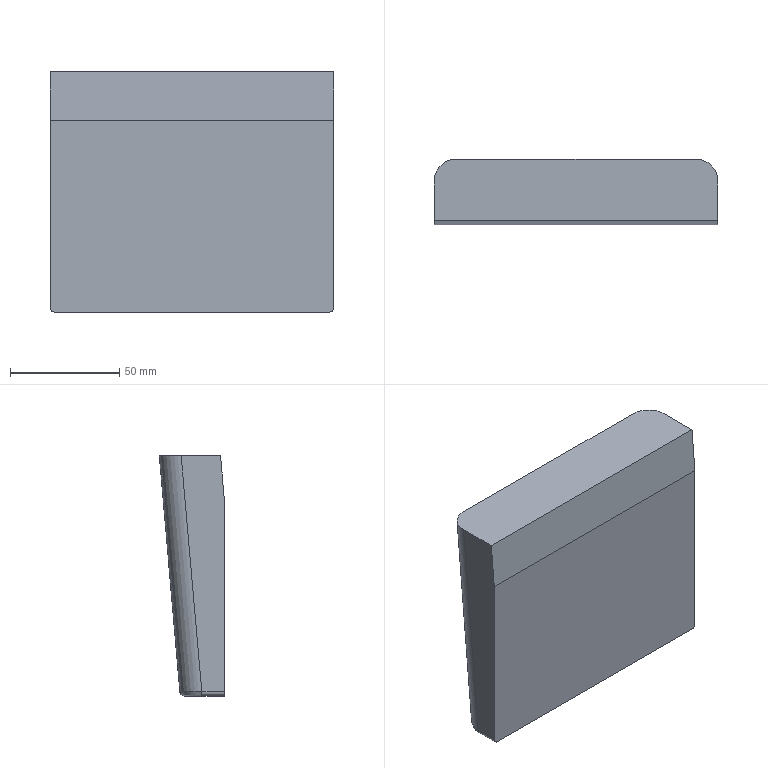Part | STEP file | 4-20.sldasm-Part-379 | 1 solid | 14 faces | box 130 x 29.992 x 110 mm | volume 352459 mm3 | plane 7 | cylinder 5 | spline 2 | commonest cylinder face diameters 4 x3 20 x2
STEP:
#1=CARTESIAN_POINT('',(65.,431.929,150.));
#2=VERTEX_POINT('',#1);
#3=CARTESIAN_POINT('',(65.,449.954,150.));
#4=VERTEX_POINT('',#3);
#5=CARTESIAN_POINT('',(65.,430.,150.));
#6=DIRECTION('',(0.,1.,0.));
#7=VECTOR('',#6,1000.);
#8=LINE('',#5,#7);
#9=EDGE_CURVE('',#2,#4,#8,.T.);
#10=ORIENTED_EDGE('',*,*,#9,.F.);
#11=CARTESIAN_POINT('',(65.,430.,127.947));
#12=VERTEX_POINT('',#11);
#13=CARTESIAN_POINT('',(65.,440.597,249.073));
#14=DIRECTION('',(0.,-0.08716,-0.9962));
#15=VECTOR('',#14,1000.);
#16=LINE('',#13,#15);
#17=EDGE_CURVE('',#2,#12,#16,.T.);
#18=ORIENTED_EDGE('',*,*,#17,.T.);
#19=CARTESIAN_POINT('',(65.,430.,42.));
#20=VERTEX_POINT('',#19);
#21=CARTESIAN_POINT('',(65.,430.,250.));
#22=DIRECTION('',(0.,0.,-1.));
#23=VECTOR('',#22,1000.);
#24=LINE('',#21,#23);
#25=EDGE_CURVE('',#12,#20,#24,.T.);
#26=ORIENTED_EDGE('',*,*,#25,.T.);
#27=CARTESIAN_POINT('',(65.,440.505,42.));
#28=VERTEX_POINT('',#27);
#29=CARTESIAN_POINT('',(65.,430.,42.));
#30=DIRECTION('',(0.,1.,0.));
#31=VECTOR('',#30,1000.);
#32=LINE('',#29,#31);
#33=EDGE_CURVE('',#20,#28,#32,.T.);
#34=ORIENTED_EDGE('',*,*,#33,.T.);
#35=CARTESIAN_POINT('',(65.,458.485,247.508));
#36=DIRECTION('',(0.,0.08716,0.9962));
#37=VECTOR('',#36,1000.);
#38=LINE('',#35,#37);
#39=EDGE_CURVE('',#28,#4,#38,.T.);
#40=ORIENTED_EDGE('',*,*,#39,.T.);
#41=EDGE_LOOP('',(#10,#18,#26,#34,#40));
#42=FACE_OUTER_BOUND('',#41,.T.);
#43=CARTESIAN_POINT('',(65.,430.,250.));
#44=DIRECTION('',(-1.,0.,0.));
#45=DIRECTION('',(0.,0.,1.));
#46=AXIS2_PLACEMENT_3D('',#43,#44,#45);
#47=PLANE('',#46);
#48=ADVANCED_FACE('',(#42),#47,.F.);
#49=CARTESIAN_POINT('',(55.,459.992,150.));
#50=VERTEX_POINT('',#49);
#51=CARTESIAN_POINT('',(55.,450.528,41.826));
#52=VERTEX_POINT('',#51);
#53=CARTESIAN_POINT('',(55.,460.008,150.174));
#54=DIRECTION('',(0.,-0.08716,-0.9962));
#55=VECTOR('',#54,1000.);
#56=LINE('',#53,#55);
#57=EDGE_CURVE('',#50,#52,#56,.T.);
#58=ORIENTED_EDGE('',*,*,#57,.T.);
#59=CARTESIAN_POINT('',(-55.,450.528,41.826));
#60=VERTEX_POINT('',#59);
#61=CARTESIAN_POINT('',(55.,450.528,41.826));
#62=DIRECTION('',(-1.,0.,0.));
#63=VECTOR('',#62,1000.);
#64=LINE('',#61,#63);
#65=EDGE_CURVE('',#52,#60,#64,.T.);
#66=ORIENTED_EDGE('',*,*,#65,.T.);
#67=CARTESIAN_POINT('',(-55.,459.992,150.));
#68=VERTEX_POINT('',#67);
#69=CARTESIAN_POINT('',(-55.,460.008,150.174));
#70=DIRECTION('',(0.,0.08716,0.9962));
#71=VECTOR('',#70,1000.);
#72=LINE('',#69,#71);
#73=EDGE_CURVE('',#60,#68,#72,.T.);
#74=ORIENTED_EDGE('',*,*,#73,.T.);
#75=CARTESIAN_POINT('',(55.,459.992,150.));
#76=DIRECTION('',(-1.,0.,0.));
#77=VECTOR('',#76,1000.);
#78=LINE('',#75,#77);
#79=EDGE_CURVE('',#50,#68,#78,.T.);
#80=ORIENTED_EDGE('',*,*,#79,.F.);
#81=EDGE_LOOP('',(#58,#66,#74,#80));
#82=FACE_OUTER_BOUND('',#81,.T.);
#83=CARTESIAN_POINT('',(55.,460.008,150.174));
#84=DIRECTION('',(0.,-0.9962,0.08716));
#85=DIRECTION('',(0.,-0.08716,-0.9962));
#86=AXIS2_PLACEMENT_3D('',#83,#84,#85);
#87=PLANE('',#86);
#88=ADVANCED_FACE('',(#82),#87,.F.);
#89=CARTESIAN_POINT('',(-65.,430.,127.947));
#90=VERTEX_POINT('',#89);
#91=CARTESIAN_POINT('',(-65.,430.,42.));
#92=VERTEX_POINT('',#91);
#93=CARTESIAN_POINT('',(-65.,430.,250.));
#94=DIRECTION('',(0.,0.,-1.));
#95=VECTOR('',#94,1000.);
#96=LINE('',#93,#95);
#97=EDGE_CURVE('',#90,#92,#96,.T.);
#98=ORIENTED_EDGE('',*,*,#97,.F.);
#99=CARTESIAN_POINT('',(-65.,431.929,150.));
#100=VERTEX_POINT('',#99);
#101=CARTESIAN_POINT('',(-65.,440.764,250.983));
#102=DIRECTION('',(0.,0.08716,0.9962));
#103=VECTOR('',#102,1000.);
#104=LINE('',#101,#103);
#105=EDGE_CURVE('',#90,#100,#104,.T.);
#106=ORIENTED_EDGE('',*,*,#105,.T.);
#107=CARTESIAN_POINT('',(-65.,449.954,150.));
#108=VERTEX_POINT('',#107);
#109=CARTESIAN_POINT('',(-65.,452.,150.));
#110=DIRECTION('',(0.,-1.,0.));
#111=VECTOR('',#110,1000.);
#112=LINE('',#109,#111);
#113=EDGE_CURVE('',#108,#100,#112,.T.);
#114=ORIENTED_EDGE('',*,*,#113,.F.);
#115=CARTESIAN_POINT('',(-65.,440.505,42.));
#116=VERTEX_POINT('',#115);
#117=CARTESIAN_POINT('',(-65.,458.652,249.418));
#118=DIRECTION('',(0.,-0.08716,-0.9962));
#119=VECTOR('',#118,1000.);
#120=LINE('',#117,#119);
#121=EDGE_CURVE('',#108,#116,#120,.T.);
#122=ORIENTED_EDGE('',*,*,#121,.T.);
#123=CARTESIAN_POINT('',(-65.,452.,42.));
#124=DIRECTION('',(0.,-1.,0.));
#125=VECTOR('',#124,1000.);
#126=LINE('',#123,#125);
#127=EDGE_CURVE('',#116,#92,#126,.T.);
#128=ORIENTED_EDGE('',*,*,#127,.T.);
#129=EDGE_LOOP('',(#98,#106,#114,#122,#128));
#130=FACE_OUTER_BOUND('',#129,.T.);
#131=CARTESIAN_POINT('',(-65.,452.,250.));
#132=DIRECTION('',(1.,0.,0.));
#133=DIRECTION('',(0.,0.,-1.));
#134=AXIS2_PLACEMENT_3D('',#131,#132,#133);
#135=PLANE('',#134);
#136=ADVANCED_FACE('',(#130),#135,.F.);
#137=ORIENTED_EDGE('',*,*,#25,.F.);
#138=CARTESIAN_POINT('',(-65.,430.,127.947));
#139=DIRECTION('',(-1.,0.,0.));
#140=VECTOR('',#139,1000.);
#141=LINE('',#138,#140);
#142=EDGE_CURVE('',#12,#90,#141,.T.);
#143=ORIENTED_EDGE('',*,*,#142,.T.);
#144=ORIENTED_EDGE('',*,*,#97,.T.);
#145=CARTESIAN_POINT('',(-63.,430.,40.));
#146=VERTEX_POINT('',#145);
#147=CARTESIAN_POINT('',(-63.,430.,42.));
#148=DIRECTION('',(0.,-1.,0.));
#149=DIRECTION('',(0.,0.,1.));
#150=AXIS2_PLACEMENT_3D('',#147,#148,#149);
#151=CIRCLE('',#150,2.);
#152=EDGE_CURVE('',#92,#146,#151,.T.);
#153=ORIENTED_EDGE('',*,*,#152,.T.);
#154=CARTESIAN_POINT('',(63.,430.,40.));
#155=VERTEX_POINT('',#154);
#156=CARTESIAN_POINT('',(-65.,430.,40.));
#157=DIRECTION('',(1.,0.,0.));
#158=VECTOR('',#157,1000.);
#159=LINE('',#156,#158);
#160=EDGE_CURVE('',#146,#155,#159,.T.);
#161=ORIENTED_EDGE('',*,*,#160,.T.);
#162=CARTESIAN_POINT('',(63.,430.,42.));
#163=DIRECTION('',(0.,-1.,0.));
#164=DIRECTION('',(0.,0.,1.));
#165=AXIS2_PLACEMENT_3D('',#162,#163,#164);
#166=CIRCLE('',#165,2.);
#167=EDGE_CURVE('',#155,#20,#166,.T.);
#168=ORIENTED_EDGE('',*,*,#167,.T.);
#169=EDGE_LOOP('',(#137,#143,#144,#153,#161,#168));
#170=FACE_OUTER_BOUND('',#169,.T.);
#171=CARTESIAN_POINT('',(-65.,430.,250.));
#172=DIRECTION('',(0.,1.,0.));
#173=DIRECTION('',(0.,0.,1.));
#174=AXIS2_PLACEMENT_3D('',#171,#172,#173);
#175=PLANE('',#174);
#176=ADVANCED_FACE('',(#170),#175,.F.);
#177=CARTESIAN_POINT('',(95.,431.929,150.));
#178=DIRECTION('',(-1.,0.,0.));
#179=VECTOR('',#178,1000.);
#180=LINE('',#177,#179);
#181=EDGE_CURVE('',#2,#100,#180,.T.);
#182=ORIENTED_EDGE('',*,*,#181,.F.);
#183=ORIENTED_EDGE('',*,*,#9,.T.);
#184=CARTESIAN_POINT('',(65.,449.954,150.));
#185=CARTESIAN_POINT('',(65.,455.834,150.));
#186=CARTESIAN_POINT('',(60.858,459.992,150.));
#187=CARTESIAN_POINT('',(55.,459.992,150.));
#188=(BOUNDED_CURVE()B_SPLINE_CURVE(3,(#184,#185,#186,#187),.UNSPECIFIED.,.F.,.T.)B_SPLINE_CURVE_WITH_KNOTS((4,4),(1.571,3.142),.UNSPECIFIED.)CURVE()GEOMETRIC_REPRESENTATION_ITEM()RATIONAL_B_SPLINE_CURVE((1.,0.8047,0.8047,1.))REPRESENTATION_ITEM(''));
#189=EDGE_CURVE('',#4,#50,#188,.T.);
#190=ORIENTED_EDGE('',*,*,#189,.T.);
#191=ORIENTED_EDGE('',*,*,#79,.T.);
#192=CARTESIAN_POINT('',(-55.,459.992,150.));
#193=CARTESIAN_POINT('',(-60.858,459.992,150.));
#194=CARTESIAN_POINT('',(-65.,455.834,150.));
#195=CARTESIAN_POINT('',(-65.,449.954,150.));
#196=(BOUNDED_CURVE()B_SPLINE_CURVE(3,(#192,#193,#194,#195),.UNSPECIFIED.,.F.,.F.)B_SPLINE_CURVE_WITH_KNOTS((4,4),(3.142,4.712),.UNSPECIFIED.)CURVE()GEOMETRIC_REPRESENTATION_ITEM()RATIONAL_B_SPLINE_CURVE((1.,0.8047,0.8047,1.))REPRESENTATION_ITEM(''));
#197=EDGE_CURVE('',#68,#108,#196,.T.);
#198=ORIENTED_EDGE('',*,*,#197,.T.);
#199=ORIENTED_EDGE('',*,*,#113,.T.);
#200=EDGE_LOOP('',(#182,#183,#190,#191,#198,#199));
#201=FACE_OUTER_BOUND('',#200,.T.);
#202=CARTESIAN_POINT('',(-100.,17.,150.));
#203=DIRECTION('',(0.,0.,-1.));
#204=DIRECTION('',(-1.,0.,0.));
#205=AXIS2_PLACEMENT_3D('',#202,#203,#204);
#206=PLANE('',#205);
#207=ADVANCED_FACE('',(#201),#206,.F.);
#208=CARTESIAN_POINT('',(55.,448.536,40.));
#209=VERTEX_POINT('',#208);
#210=CARTESIAN_POINT('',(63.,440.505,40.));
#211=VERTEX_POINT('',#210);
#212=CARTESIAN_POINT('',(55.,448.536,40.));
#213=CARTESIAN_POINT('',(59.686,448.536,40.));
#214=CARTESIAN_POINT('',(63.,445.21,40.));
#215=CARTESIAN_POINT('',(63.,440.505,40.));
#216=(BOUNDED_CURVE()B_SPLINE_CURVE(3,(#212,#213,#214,#215),.UNSPECIFIED.,.F.,.T.)B_SPLINE_CURVE_WITH_KNOTS((4,4),(3.142,4.712),.UNSPECIFIED.)CURVE()GEOMETRIC_REPRESENTATION_ITEM()RATIONAL_B_SPLINE_CURVE((1.,0.8047,0.8047,1.))REPRESENTATION_ITEM(''));
#217=EDGE_CURVE('',#209,#211,#216,.T.);
#218=ORIENTED_EDGE('',*,*,#217,.T.);
#219=CARTESIAN_POINT('',(63.,17.,40.));
#220=DIRECTION('',(0.,-1.,0.));
#221=VECTOR('',#220,1000.);
#222=LINE('',#219,#221);
#223=EDGE_CURVE('',#211,#155,#222,.T.);
#224=ORIENTED_EDGE('',*,*,#223,.T.);
#225=ORIENTED_EDGE('',*,*,#160,.F.);
#226=CARTESIAN_POINT('',(-63.,440.505,40.));
#227=VERTEX_POINT('',#226);
#228=CARTESIAN_POINT('',(-63.,17.,40.));
#229=DIRECTION('',(0.,1.,0.));
#230=VECTOR('',#229,1000.);
#231=LINE('',#228,#230);
#232=EDGE_CURVE('',#146,#227,#231,.T.);
#233=ORIENTED_EDGE('',*,*,#232,.T.);
#234=CARTESIAN_POINT('',(-55.,448.536,40.));
#235=VERTEX_POINT('',#234);
#236=CARTESIAN_POINT('',(-63.,440.505,40.));
#237=CARTESIAN_POINT('',(-63.,445.21,40.));
#238=CARTESIAN_POINT('',(-59.686,448.536,40.));
#239=CARTESIAN_POINT('',(-55.,448.536,40.));
#240=(BOUNDED_CURVE()B_SPLINE_CURVE(3,(#236,#237,#238,#239),.UNSPECIFIED.,.F.,.F.)B_SPLINE_CURVE_WITH_KNOTS((4,4),(1.571,3.142),.UNSPECIFIED.)CURVE()GEOMETRIC_REPRESENTATION_ITEM()RATIONAL_B_SPLINE_CURVE((1.,0.8047,0.8047,1.))REPRESENTATION_ITEM(''));
#241=EDGE_CURVE('',#227,#235,#240,.T.);
#242=ORIENTED_EDGE('',*,*,#241,.T.);
#243=CARTESIAN_POINT('',(100.,448.536,40.));
#244=DIRECTION('',(1.,0.,0.));
#245=VECTOR('',#244,1000.);
#246=LINE('',#243,#245);
#247=EDGE_CURVE('',#235,#209,#246,.T.);
#248=ORIENTED_EDGE('',*,*,#247,.T.);
#249=EDGE_LOOP('',(#218,#224,#225,#233,#242,#248));
#250=FACE_OUTER_BOUND('',#249,.T.);
#251=CARTESIAN_POINT('',(100.,17.,40.));
#252=DIRECTION('',(0.,0.,-1.));
#253=DIRECTION('',(-1.,0.,0.));
#254=AXIS2_PLACEMENT_3D('',#251,#252,#253);
#255=PLANE('',#254);
#256=ADVANCED_FACE('',(#250),#255,.T.);
#257=ORIENTED_EDGE('',*,*,#73,.F.);
#258=CARTESIAN_POINT('',(-55.,450.528,41.826));
#259=CARTESIAN_POINT('',(-60.858,450.528,41.826));
#260=CARTESIAN_POINT('',(-65.,446.377,41.898));
#261=CARTESIAN_POINT('',(-65.,440.505,42.));
#262=(BOUNDED_CURVE()B_SPLINE_CURVE(3,(#258,#259,#260,#261),.UNSPECIFIED.,.F.,.T.)B_SPLINE_CURVE_WITH_KNOTS((4,4),(3.142,4.712),.UNSPECIFIED.)CURVE()GEOMETRIC_REPRESENTATION_ITEM()RATIONAL_B_SPLINE_CURVE((1.,0.8047,0.8047,1.))REPRESENTATION_ITEM(''));
#263=EDGE_CURVE('',#60,#116,#262,.T.);
#264=ORIENTED_EDGE('',*,*,#263,.T.);
#265=ORIENTED_EDGE('',*,*,#121,.F.);
#266=ORIENTED_EDGE('',*,*,#197,.F.);
#267=EDGE_LOOP('',(#257,#264,#265,#266));
#268=FACE_OUTER_BOUND('',#267,.T.);
#269=CARTESIAN_POINT('',(-55.,458.652,249.418));
#270=DIRECTION('',(0.,-0.08716,-0.9962));
#271=DIRECTION('',(0.,0.9962,-0.08716));
#272=AXIS2_PLACEMENT_3D('',#269,#270,#271);
#273=CYLINDRICAL_SURFACE('',#272,10.);
#274=ADVANCED_FACE('',(#268),#273,.T.);
#275=ORIENTED_EDGE('',*,*,#39,.F.);
#276=CARTESIAN_POINT('',(65.,440.505,42.));
#277=CARTESIAN_POINT('',(65.,446.377,41.898));
#278=CARTESIAN_POINT('',(60.858,450.528,41.826));
#279=CARTESIAN_POINT('',(55.,450.528,41.826));
#280=(BOUNDED_CURVE()B_SPLINE_CURVE(3,(#276,#277,#278,#279),.UNSPECIFIED.,.F.,.F.)B_SPLINE_CURVE_WITH_KNOTS((4,4),(1.571,3.142),.UNSPECIFIED.)CURVE()GEOMETRIC_REPRESENTATION_ITEM()RATIONAL_B_SPLINE_CURVE((1.,0.8047,0.8047,1.))REPRESENTATION_ITEM(''));
#281=EDGE_CURVE('',#28,#52,#280,.T.);
#282=ORIENTED_EDGE('',*,*,#281,.T.);
#283=ORIENTED_EDGE('',*,*,#57,.F.);
#284=ORIENTED_EDGE('',*,*,#189,.F.);
#285=EDGE_LOOP('',(#275,#282,#283,#284));
#286=FACE_OUTER_BOUND('',#285,.T.);
#287=CARTESIAN_POINT('',(55.,450.046,151.046));
#288=DIRECTION('',(0.,-0.08716,-0.9962));
#289=DIRECTION('',(0.,0.9962,-0.08716));
#290=AXIS2_PLACEMENT_3D('',#287,#288,#289);
#291=CYLINDRICAL_SURFACE('',#290,10.);
#292=ADVANCED_FACE('',(#286),#291,.T.);
#293=ORIENTED_EDGE('',*,*,#152,.F.);
#294=ORIENTED_EDGE('',*,*,#127,.F.);
#295=CARTESIAN_POINT('',(-63.,440.505,42.));
#296=DIRECTION('',(0.,1.,0.));
#297=DIRECTION('',(0.,0.,1.));
#298=AXIS2_PLACEMENT_3D('',#295,#296,#297);
#299=CIRCLE('',#298,2.);
#300=EDGE_CURVE('',#227,#116,#299,.T.);
#301=ORIENTED_EDGE('',*,*,#300,.F.);
#302=ORIENTED_EDGE('',*,*,#232,.F.);
#303=EDGE_LOOP('',(#293,#294,#301,#302));
#304=FACE_OUTER_BOUND('',#303,.T.);
#305=CARTESIAN_POINT('',(-63.,452.,42.));
#306=DIRECTION('',(0.,1.,0.));
#307=DIRECTION('',(0.,0.,1.));
#308=AXIS2_PLACEMENT_3D('',#305,#306,#307);
#309=CYLINDRICAL_SURFACE('',#308,2.);
#310=ADVANCED_FACE('',(#304),#309,.T.);
#311=ORIENTED_EDGE('',*,*,#300,.T.);
#312=ORIENTED_EDGE('',*,*,#263,.F.);
#313=CARTESIAN_POINT('',(-55.,448.536,42.));
#314=DIRECTION('',(1.,0.,0.));
#315=DIRECTION('',(0.,0.,-1.));
#316=AXIS2_PLACEMENT_3D('',#313,#314,#315);
#317=CIRCLE('',#316,2.);
#318=EDGE_CURVE('',#235,#60,#317,.T.);
#319=ORIENTED_EDGE('',*,*,#318,.F.);
#320=ORIENTED_EDGE('',*,*,#241,.F.);
#321=EDGE_LOOP('',(#311,#312,#319,#320));
#322=FACE_OUTER_BOUND('',#321,.T.);
#323=CARTESIAN_POINT('',(-65.,440.505,42.));
#324=CARTESIAN_POINT('',(-65.,440.505,40.));
#325=CARTESIAN_POINT('',(-63.,440.505,40.));
#326=CARTESIAN_POINT('',(-65.,441.818,41.977));
#327=CARTESIAN_POINT('',(-64.977,441.81,40.));
#328=CARTESIAN_POINT('',(-63.,441.557,40.));
#329=CARTESIAN_POINT('',(-64.74,443.129,41.954));
#330=CARTESIAN_POINT('',(-64.698,443.113,40.));
#331=CARTESIAN_POINT('',(-62.792,442.607,40.));
#332=CARTESIAN_POINT('',(-63.738,445.553,41.912));
#333=CARTESIAN_POINT('',(-63.666,445.507,40.));
#334=CARTESIAN_POINT('',(-61.99,444.55,40.));
#335=CARTESIAN_POINT('',(-62.997,446.665,41.893));
#336=CARTESIAN_POINT('',(-62.917,446.601,40.));
#337=CARTESIAN_POINT('',(-61.397,445.441,40.));
#338=CARTESIAN_POINT('',(-61.145,448.52,41.861));
#339=CARTESIAN_POINT('',(-61.067,448.414,40.));
#340=CARTESIAN_POINT('',(-59.916,446.927,40.));
#341=CARTESIAN_POINT('',(-60.036,449.263,41.848));
#342=CARTESIAN_POINT('',(-59.966,449.139,40.));
#343=CARTESIAN_POINT('',(-59.029,447.522,40.));
#344=CARTESIAN_POINT('',(-57.617,450.267,41.83));
#345=CARTESIAN_POINT('',(-57.578,450.115,40.));
#346=CARTESIAN_POINT('',(-57.094,448.327,40.));
#347=CARTESIAN_POINT('',(-56.309,450.528,41.826));
#348=CARTESIAN_POINT('',(-56.288,450.369,40.));
#349=CARTESIAN_POINT('',(-56.047,448.536,40.));
#350=CARTESIAN_POINT('',(-55.,450.528,41.826));
#351=CARTESIAN_POINT('',(-55.,450.369,40.));
#352=CARTESIAN_POINT('',(-55.,448.536,40.));
#353=(BOUNDED_SURFACE()B_SPLINE_SURFACE(3,2,((#323,#324,#325),(#326,#327,#328),(#329,#330,#331),(#332,#333,#334),(#335,#336,#337),(#338,#339,#340),(#341,#342,#343),(#344,#345,#346),(#347,#348,#349),(#350,#351,#352)),.UNSPECIFIED.,.F.,.F.,.T.)B_SPLINE_SURFACE_WITH_KNOTS((4,2,2,2,4),(3,3),(1.571,1.963,2.356,2.749,3.142),(0.,1.),.UNSPECIFIED.)GEOMETRIC_REPRESENTATION_ITEM()RATIONAL_B_SPLINE_SURFACE(((1.,0.7071,1.),(1.,0.7111,1.),(1.,0.7151,1.),(1.,0.7225,1.),(1.,0.7258,1.),(1.,0.7313,1.),(1.,0.7335,1.),(1.,0.7365,1.),(1.,0.7373,1.),(1.,0.7373,1.)))REPRESENTATION_ITEM('')SURFACE());
#354=ADVANCED_FACE('',(#322),#353,.T.);
#355=ORIENTED_EDGE('',*,*,#318,.T.);
#356=ORIENTED_EDGE('',*,*,#65,.F.);
#357=CARTESIAN_POINT('',(55.,448.536,42.));
#358=DIRECTION('',(1.,0.,0.));
#359=DIRECTION('',(0.,0.,-1.));
#360=AXIS2_PLACEMENT_3D('',#357,#358,#359);
#361=CIRCLE('',#360,2.);
#362=EDGE_CURVE('',#209,#52,#361,.T.);
#363=ORIENTED_EDGE('',*,*,#362,.F.);
#364=ORIENTED_EDGE('',*,*,#247,.F.);
#365=EDGE_LOOP('',(#355,#356,#363,#364));
#366=FACE_OUTER_BOUND('',#365,.T.);
#367=CARTESIAN_POINT('',(55.,448.536,42.));
#368=DIRECTION('',(1.,0.,0.));
#369=DIRECTION('',(0.,1.,0.));
#370=AXIS2_PLACEMENT_3D('',#367,#368,#369);
#371=CYLINDRICAL_SURFACE('',#370,2.);
#372=ADVANCED_FACE('',(#366),#371,.T.);
#373=ORIENTED_EDGE('',*,*,#362,.T.);
#374=ORIENTED_EDGE('',*,*,#281,.F.);
#375=CARTESIAN_POINT('',(63.,440.505,42.));
#376=DIRECTION('',(0.,-1.,0.));
#377=DIRECTION('',(0.,0.,-1.));
#378=AXIS2_PLACEMENT_3D('',#375,#376,#377);
#379=CIRCLE('',#378,2.);
#380=EDGE_CURVE('',#211,#28,#379,.T.);
#381=ORIENTED_EDGE('',*,*,#380,.F.);
#382=ORIENTED_EDGE('',*,*,#217,.F.);
#383=EDGE_LOOP('',(#373,#374,#381,#382));
#384=FACE_OUTER_BOUND('',#383,.T.);
#385=CARTESIAN_POINT('',(55.,450.528,41.826));
#386=CARTESIAN_POINT('',(55.,450.369,40.));
#387=CARTESIAN_POINT('',(55.,448.536,40.));
#388=CARTESIAN_POINT('',(56.309,450.528,41.826));
#389=CARTESIAN_POINT('',(56.288,450.369,40.));
#390=CARTESIAN_POINT('',(56.047,448.536,40.));
#391=CARTESIAN_POINT('',(57.617,450.267,41.83));
#392=CARTESIAN_POINT('',(57.578,450.115,40.));
#393=CARTESIAN_POINT('',(57.094,448.327,40.));
#394=CARTESIAN_POINT('',(60.036,449.263,41.848));
#395=CARTESIAN_POINT('',(59.966,449.139,40.));
#396=CARTESIAN_POINT('',(59.029,447.522,40.));
#397=CARTESIAN_POINT('',(61.145,448.52,41.861));
#398=CARTESIAN_POINT('',(61.067,448.414,40.));
#399=CARTESIAN_POINT('',(59.916,446.927,40.));
#400=CARTESIAN_POINT('',(62.997,446.665,41.893));
#401=CARTESIAN_POINT('',(62.917,446.601,40.));
#402=CARTESIAN_POINT('',(61.397,445.441,40.));
#403=CARTESIAN_POINT('',(63.738,445.553,41.912));
#404=CARTESIAN_POINT('',(63.666,445.507,40.));
#405=CARTESIAN_POINT('',(61.99,444.55,40.));
#406=CARTESIAN_POINT('',(64.74,443.129,41.954));
#407=CARTESIAN_POINT('',(64.698,443.113,40.));
#408=CARTESIAN_POINT('',(62.792,442.607,40.));
#409=CARTESIAN_POINT('',(65.,441.818,41.977));
#410=CARTESIAN_POINT('',(64.977,441.81,40.));
#411=CARTESIAN_POINT('',(63.,441.557,40.));
#412=CARTESIAN_POINT('',(65.,440.505,42.));
#413=CARTESIAN_POINT('',(65.,440.505,40.));
#414=CARTESIAN_POINT('',(63.,440.505,40.));
#415=(BOUNDED_SURFACE()B_SPLINE_SURFACE(3,2,((#385,#386,#387),(#388,#389,#390),(#391,#392,#393),(#394,#395,#396),(#397,#398,#399),(#400,#401,#402),(#403,#404,#405),(#406,#407,#408),(#409,#410,#411),(#412,#413,#414)),.UNSPECIFIED.,.F.,.F.,.F.)B_SPLINE_SURFACE_WITH_KNOTS((4,2,2,2,4),(3,3),(3.142,3.534,3.927,4.32,4.712),(0.,1.),.UNSPECIFIED.)GEOMETRIC_REPRESENTATION_ITEM()RATIONAL_B_SPLINE_SURFACE(((1.,0.7373,1.),(1.,0.7373,1.),(1.,0.7365,1.),(1.,0.7335,1.),(1.,0.7313,1.),(1.,0.7258,1.),(1.,0.7225,1.),(1.,0.7151,1.),(1.,0.7111,1.),(1.,0.7071,1.)))REPRESENTATION_ITEM('')SURFACE());
#416=ADVANCED_FACE('',(#384),#415,.T.);
#417=ORIENTED_EDGE('',*,*,#167,.F.);
#418=ORIENTED_EDGE('',*,*,#223,.F.);
#419=ORIENTED_EDGE('',*,*,#380,.T.);
#420=ORIENTED_EDGE('',*,*,#33,.F.);
#421=EDGE_LOOP('',(#417,#418,#419,#420));
#422=FACE_OUTER_BOUND('',#421,.T.);
#423=CARTESIAN_POINT('',(63.,430.,42.));
#424=DIRECTION('',(0.,-1.,0.));
#425=DIRECTION('',(0.,0.,-1.));
#426=AXIS2_PLACEMENT_3D('',#423,#424,#425);
#427=CYLINDRICAL_SURFACE('',#426,2.);
#428=ADVANCED_FACE('',(#422),#427,.T.);
#429=ORIENTED_EDGE('',*,*,#181,.T.);
#430=ORIENTED_EDGE('',*,*,#105,.F.);
#431=ORIENTED_EDGE('',*,*,#142,.F.);
#432=ORIENTED_EDGE('',*,*,#17,.F.);
#433=EDGE_LOOP('',(#429,#430,#431,#432));
#434=FACE_OUTER_BOUND('',#433,.T.);
#435=CARTESIAN_POINT('',(0.,428.008,105.174));
#436=DIRECTION('',(0.,-0.9962,0.08716));
#437=DIRECTION('',(0.,0.08716,0.9962));
#438=AXIS2_PLACEMENT_3D('',#435,#436,#437);
#439=PLANE('',#438);
#440=ADVANCED_FACE('',(#434),#439,.T.);
#441=CLOSED_SHELL('',(#48,#88,#136,#176,#207,#256,#274,#292,#310,#354,#372,#416,#428,#440));
#442=MANIFOLD_SOLID_BREP('',#441);
#443=CARTESIAN_POINT('',(0.,0.,0.));
#444=DIRECTION('',(0.,0.,1.));
#445=DIRECTION('',(1.,0.,0.));
#446=AXIS2_PLACEMENT_3D('',#443,#444,#445);
#447=(LENGTH_UNIT()NAMED_UNIT(*)SI_UNIT(.MILLI.,.METRE.));
#448=UNCERTAINTY_MEASURE_WITH_UNIT(LENGTH_MEASURE(0.00001),#447,'','');
#449=(NAMED_UNIT(*)PLANE_ANGLE_UNIT()SI_UNIT($,.RADIAN.));
#450=(NAMED_UNIT(*)SI_UNIT($,.STERADIAN.)SOLID_ANGLE_UNIT());
#451=(GEOMETRIC_REPRESENTATION_CONTEXT(3)GLOBAL_UNCERTAINTY_ASSIGNED_CONTEXT((#448))GLOBAL_UNIT_ASSIGNED_CONTEXT((#447,#449,#450))REPRESENTATION_CONTEXT('',''));
#452=ADVANCED_BREP_SHAPE_REPRESENTATION('',(#442,#446),#451);